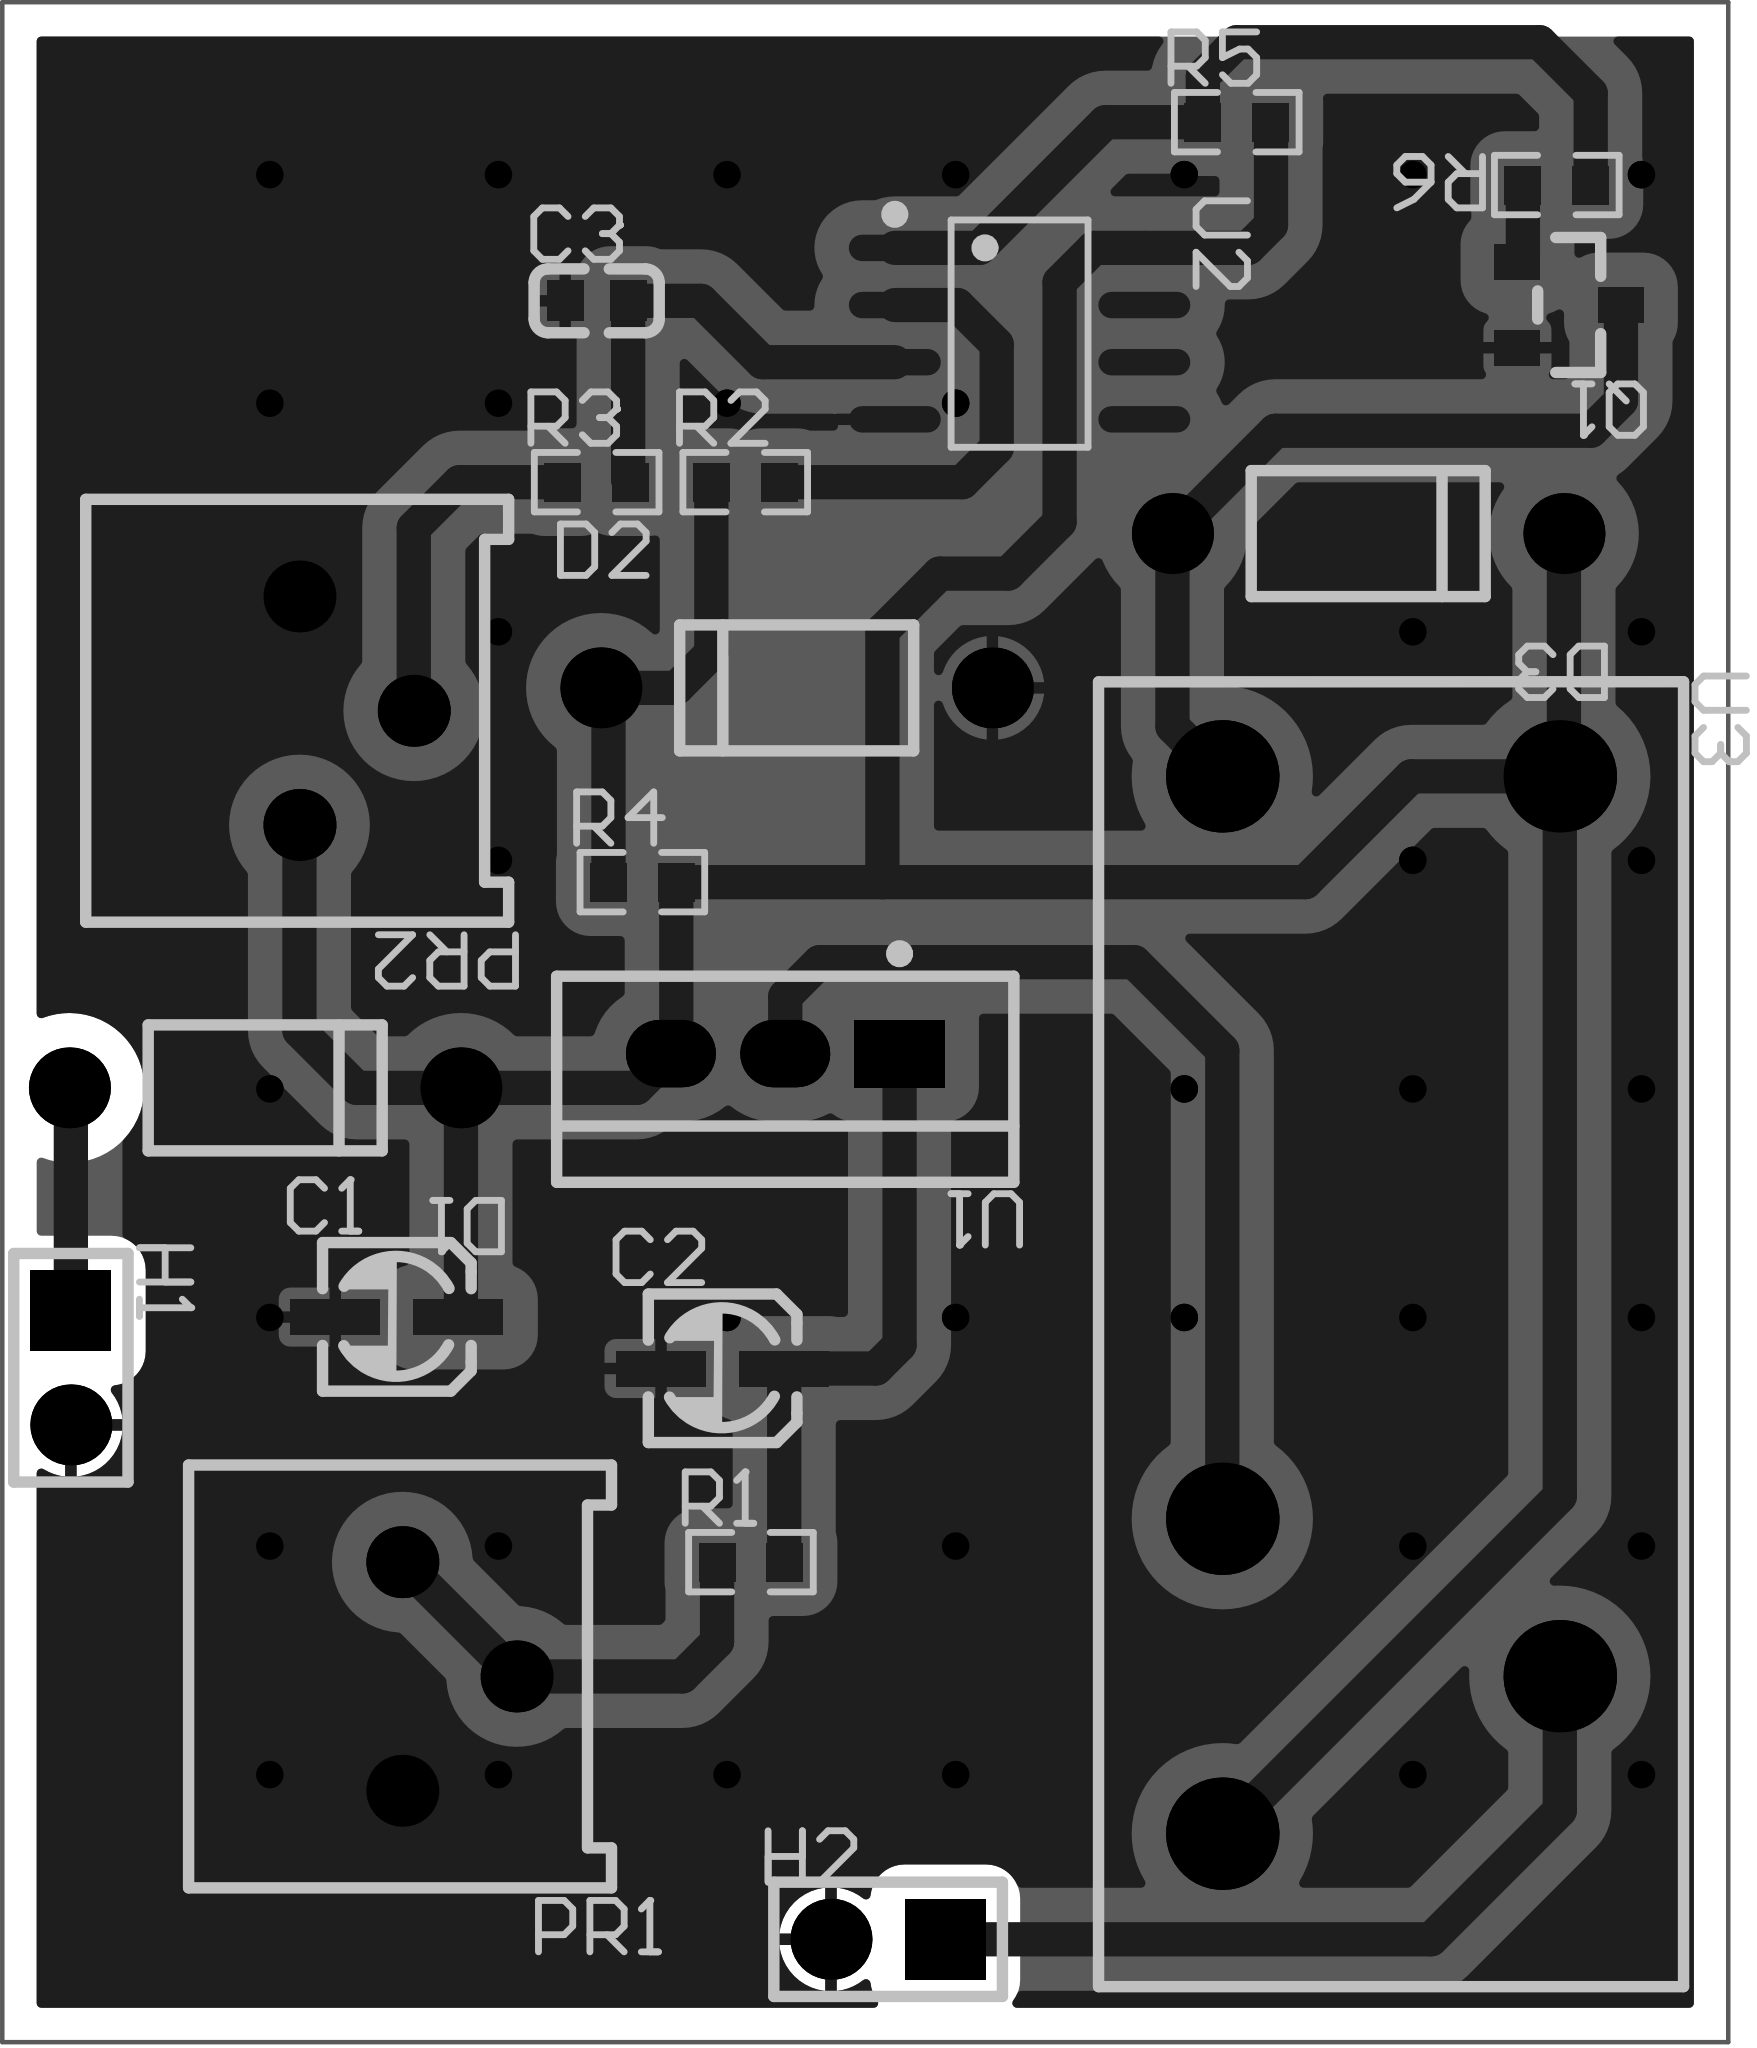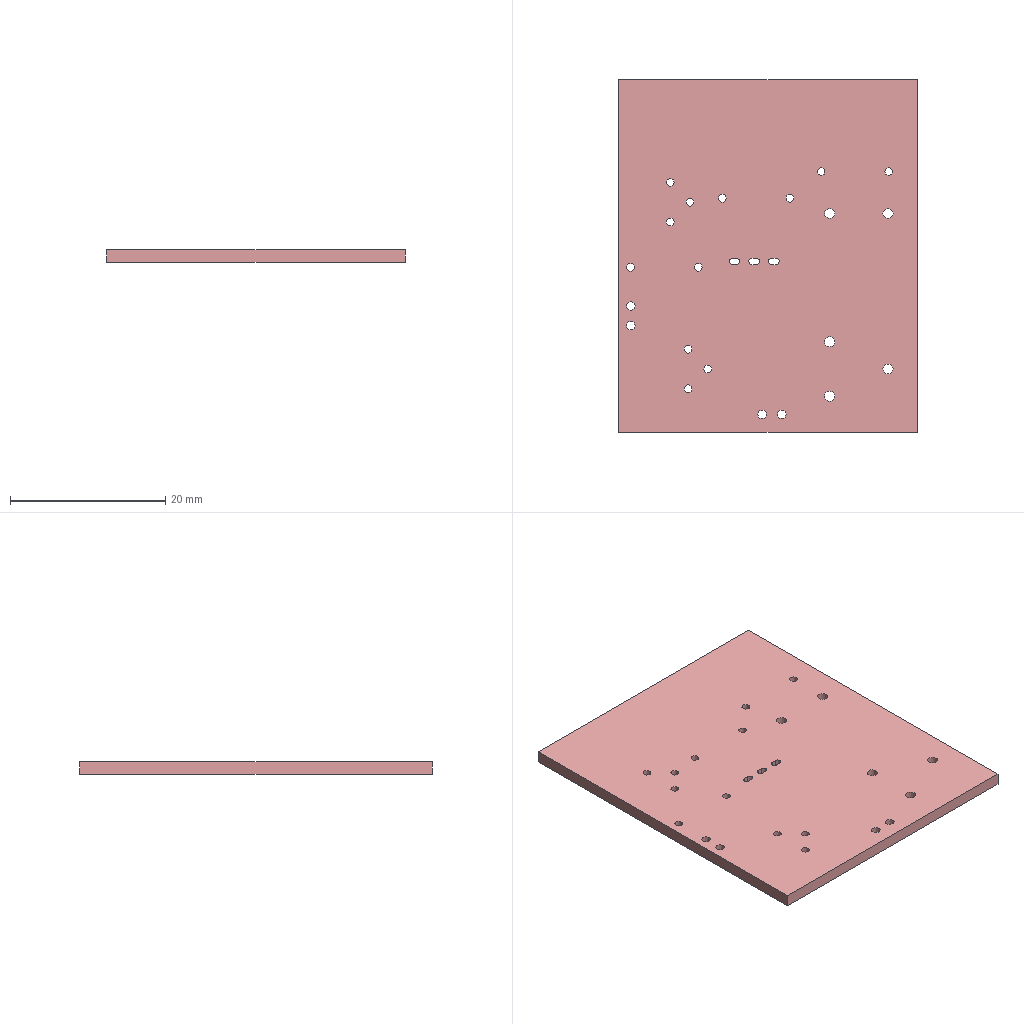Circuit board layout | Altium Designer | box 38.4 x 45.3 x 1.6 mm
Layer stack:
# Altium Designer layer stack of  (unit mm; dielectric type: 0 none, 1 core, 2 prepreg, 3 surface material)
index,name,kind,layer,copper_thickness_mm,dielectric_type,dielectric_thickness_mm,dielectric_material,dielectric_constant
0,Top Paste Mask Layer,other,,,,,,
1,Top Silkscreen Layer,other,,,,,,
2,Top Solder Mask Layer,dielectric,,,3,0.01,,3.3
3,Top Layer,copper,Top Layer,0.035,,,,
4,Dielectric1,dielectric,,,3,1.51,FR4,4.5
5,Bottom Layer,copper,Bottom Layer,0.035,,,,
6,Bottom Solder Mask Layer,dielectric,,,3,0.01,,3.3
7,Bottom Silkscreen Layer,other,,,,,,
8,Bottom Paste Mask Layer,other,,,,,,
# drill layer pairs: low layer,high layer
drill_pair,Top Layer,Bottom Layer
Part placement:
Designator,Comment,Layer,Footprint,Center-X(mm),Center-Y(mm),Rotation
C1,1uF,TopLayer,C_Ele_SMD_3x5.4mm,88.905,95.617,0
C2,10uF,TopLayer,C_Ele_SMD_3x5.4mm,96.144,94.474,0
C3,100nF,TopLayer,C0603,93.345,118.204,180
D1,,TopLayer,DO_1N4007,85.979,100.711,180
D2,,TopLayer,DO_1N4007,97.79,109.601,0
D3,,TopLayer,DO_1N4007,110.49,113.03,180
H1,,TopLayer,HDR-TH_2P-P2.54-V-M-1,81.661,94.491,270
H2,,TopLayer,HDR-TH_2P-P2.54-V-M-1,99.822,81.788,180
PR1,10K,TopLayer,R_3386P,90.297,87.63,180
PR2,200K,TopLayer,R_3386P,88.011,109.093,180
Q1,,TopLayer,S8050_SOT-23,114.957,118.111,180
R1,240,TopLayer,R0603,96.774,90.17,0
R2,4.7K,TopLayer,R0603,96.647,114.173,0
R3,4.7K,TopLayer,R0603,93.345,114.173,0
R4,4.7K,TopLayer,R0603,94.361,105.283,0
R5,10K,TopLayer,R0603,107.569,122.174,0
R6,4.7K,TopLayer,R0603,114.681,120.777,0
U1,LM317T,TopLayer,TO-220-3_L10.2-W4.6-P2.54-L,97.536,101.473,180
U2,LM393DG4,TopLayer,SOIC-8_L4.9-W3.9-P1.27-LS6.0-BL,102.743,117.475,270
U3,G2R-1 继电器座,TopLayer,RELAY-TH_G2R-1_C9900014679,110.998,95.885,270
Pad and via stacks:
# Altium Designer via and pad stacks of  (unit mm). Each distinct definition once, with the count of objects using it.
# via: kind,start_layer,end_layer,hole_mm,diameter_mm,mode(0 simple;1 top-mid-bottom;2 full stack),diameter_per_layer,count,example_net
# pad: kind,layer,hole_mm,hole_type(0 round;1 square;2 slot),plating,top_size,top_shape(1 round;2 rect;3 octagon;9 rounded rect),mid_size,bottom_size,mode,footprint,size_per_layer,count,example
pad,Top Layer,0,0,plated,1.999x0.8001,2,1.999x0.8001,1.999x0.8001,0,C_Ele_SMD_3x5.4mm,,4,C1.1
pad,Top Layer,0,0,plated,0.8x0.9,2,0.8x0.9,0.8x0.9,0,C0603,,2,C3.2
pad,Top Layer,0,0,plated,1x0.8,2,1x0.8,1x0.8,0,S8050_SOT-23,,3,Q1.2
pad,Top Layer,0,0,plated,0.8065x0.864,2,0.8065x0.864,0.8065x0.864,0,R0603,,12,R1.2
pad,Top Layer,0,0,plated,0.588x2.045,1,0.588x2.045,0.588x2.045,0,SOIC-8_L4.9-W3.9-P1.27-LS6.0-BL,,8,U2.1
pad,Multi-Layer,1,0,plated,1.8x1.8,1,1.8x1.8,1.8x1.8,0,DO_1N4007,,6,D1.1
pad,Multi-Layer,1.1,0,plated,1.8x1.8,1,1.8x1.8,1.8x1.8,0,HDR-TH_2P-P2.54-V-M-1,,2,H1.2
pad,Multi-Layer,1.1,0,plated,1.8x1.8,2,1.8x1.8,1.8x1.8,0,HDR-TH_2P-P2.54-V-M-1,,2,H1.1
pad,Multi-Layer,1.001,0,plated,1.6x1.6,1,1.6x1.6,1.6x1.6,0,R_3386P,,6,PR1.2
pad,Multi-Layer,0.8,2,plated,2x1.5,1,2x1.5,2x1.5,0,TO-220-3_L10.2-W4.6-P2.54-L,,2,U1.2
pad,Multi-Layer,0.8,2,plated,2x1.5,2,2x1.5,2x1.5,0,TO-220-3_L10.2-W4.6-P2.54-L,,1,U1.1
pad,Multi-Layer,1.3,0,plated,2.5x2.5,1,2.5x2.5,2.5x2.5,0,RELAY-TH_G2R-1_C9900014679,,5,U3.1
via,Top Layer,Bottom Layer,0.3048,0.61,0,,38,GND
Copper pours:
name,layer,net,type(0 solid;1 hatched;2 none)
Top Layer-GND,Top Layer,GND,0
Bottom Layer-GND,Bottom Layer,GND,0
Design rules, without the lines most boards share:
# Altium Designer design rules of  (exported by Altium Designer, unit mm)
# columns: name | kind | enabled | priority | scope1 | scope2 | descriptor | typed fields (field=value)
viaSize | 11 | enabled | 1 | All | All | Routing Via (MinHoleWidth=11.811mil) (MaxHoleWidth=248.032mil) (PreferredHoleWidth=12.008mil) (MinWidth=19.685mil) (MaxWidth=393.701mil) (PreferedWidth=24.016mil) (All) | via_min_hole=0.3 via_max_hole=6.3 via_preferred_diameter=0.61 via_preferred_hole=0.305
solderMaskExpansion | 13 | enabled | 2 | All | All | Solder Mask Expansion (Expansion =2.008mil) (All) | expansion=0.051